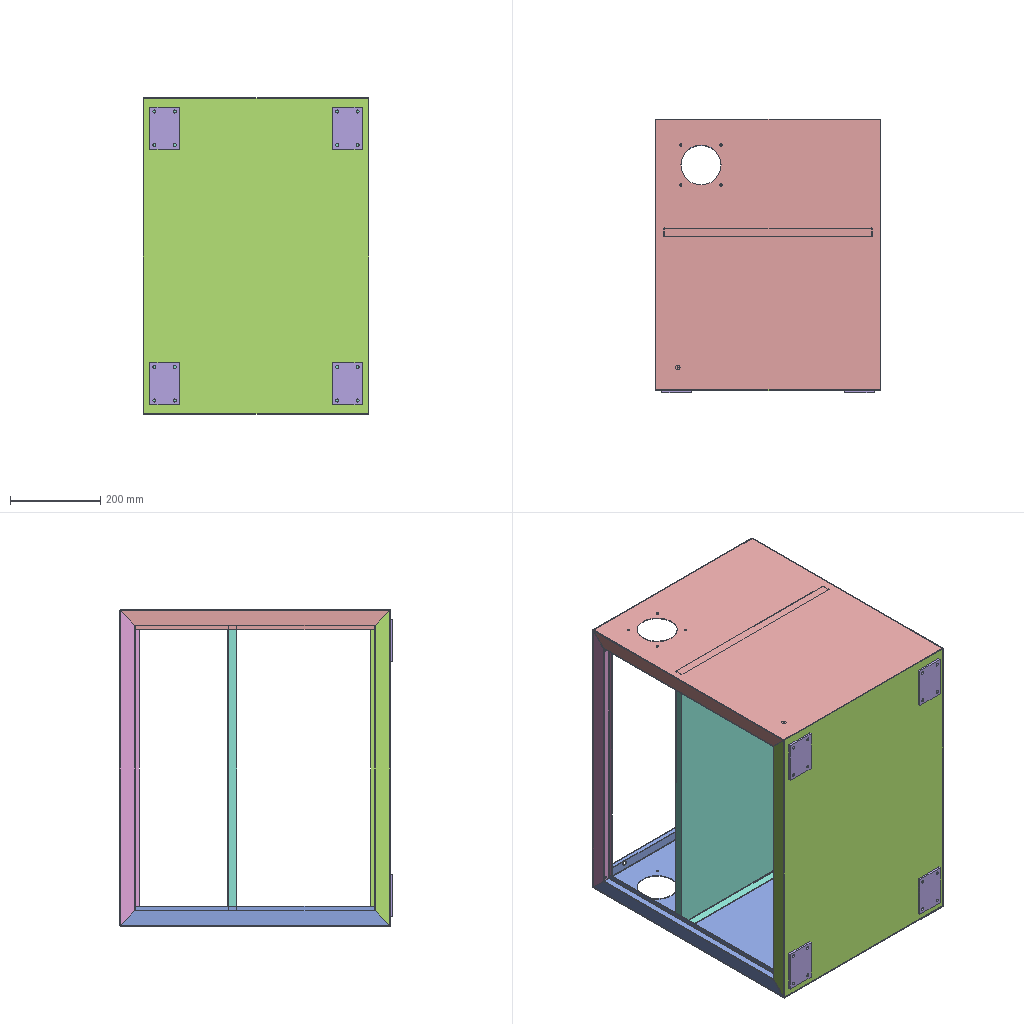Assembly | SolidWorks | 7 different items | 11 placed | box 500 x 605 x 700 mm
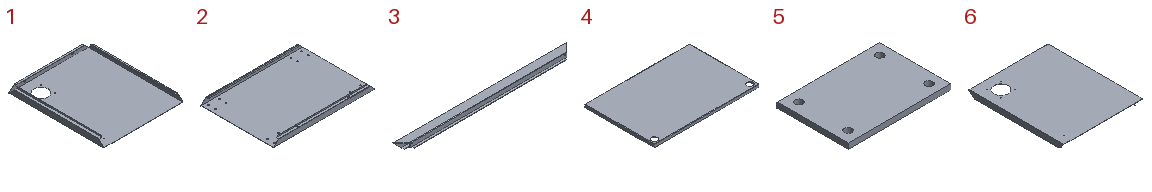Parts list (item | name | quantity | size | volume | features):
1 | - | x1 | 500 x 598.5 x 43.5 mm | 564648 mm3 | features EdgeFlange 5, ICE 3, FlatPattern 1, MirrorPattern 1, SMBaseFlange 1, SheetMetal 1
2 | - | x1 | 700 x 500 x 43.5 mm | 635964 mm3 | features EdgeFlange 3, ICE 2, FlatPattern 1, MirrorPattern 1, SMBaseFlange 1, SheetMetal 1
3 | - | x2 | 697 x 43.5 x 35 mm | 100366 mm3 | features EdgeFlange 4, ICE 2, FlatPattern 1, LPattern 1, SMBaseFlange 1, SheetMetal 1
4 | - | x1 | 697 x 463 x 20 mm | 721539 mm3 | features Extrusion 1, FlatPattern 1, FlattenBends 1, ICE 1, ProcessBends 1, Rip 1, SheetMetal 1, Shell 1
5 | - | x4 | 94 x 65 x 5 mm | 29824 mm3 | features FlatPattern 1, SMBaseFlange 1, SheetMetal 1
6 | - | x1 | 500 x 598.5 x 43.5 mm | 564648 mm3 | features EdgeFlange 5, ICE 3, FlatPattern 1, MirrorPattern 1, SMBaseFlange 1, SheetMetal 1
7 | hexagon fit bolts--product grade a and b gb | x1 | - | - | -
Mates (type | each side: item.copy, entity, surface, feature):
Coincident | 6.1 face plane Edge-Flange1 | 1.1 face plane Edge-Flange1
Coincident | 6.1 face plane Edge-Flange2 | 1.1 face plane Edge-Flange2
DistanceDim | 6.1 face plane Base-Flange1 | 1.1 face plane Base-Flange1
Coincident | 6.1 face plane Base-Flange1 | 2.1 face plane Base-Flange1 | 2 times
Coincident | 6.1 face plane Edge-Flange2 | 2.1 face plane Mirror1
Coincident | 1.1 face plane Edge-Flange1 | 3.1 face plane Edge-Flange1 | 2 times
Coincident | 1.1 face plane Edge-Flange2 | 3.1 face plane Base-Flange1
Coincident | 6.1 face plane Edge-Flange1 | 3.2 face plane Edge-Flange1 | 2 times
Coincident | 6.1 face plane Mirror1 | 3.2 face plane Base-Flange1
DistanceDim | 4.1 face plane Boss-Extrude1 | 1.1 face plane Base-Flange1
Coincident | 1.1 face plane Mirror1 | 4.1 face plane Boss-Extrude1
DistanceDim | 4.1 face plane Boss-Extrude1 | 2.1 face plane Base-Flange1
Coincident | 2.1 face plane Base-Flange1 | 5.1 face plane Base-Flange1
Concentric | 2.1 face cylinder Cut-Extrude2 | 5.1 face cylinder Base-Flange1 | 2 times